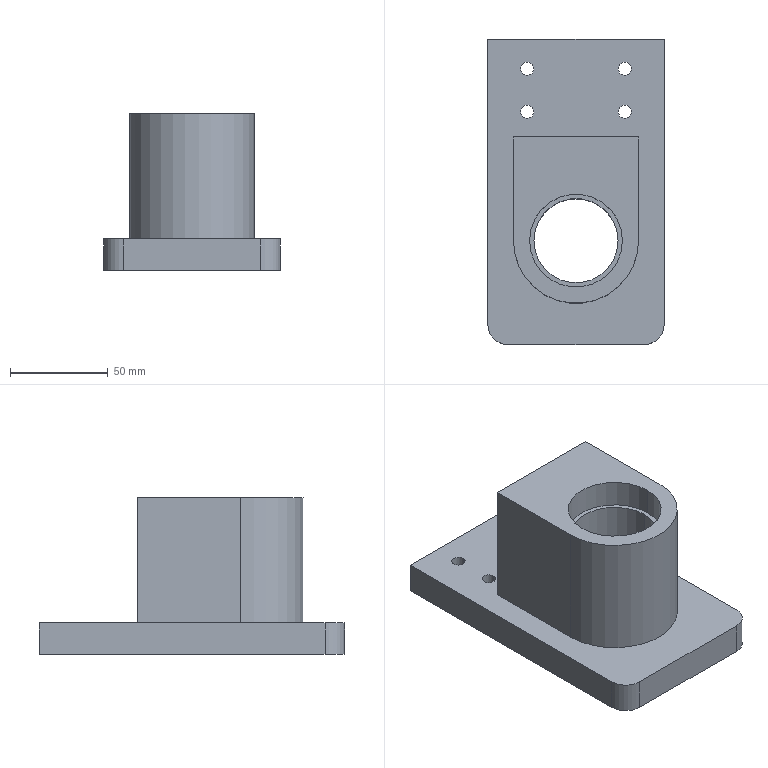NC program | NX | posted with a generic post | part box 90 x 156 x 80 mm
Lines 4809 to 4831 of 8711:
(PLANAR_MILL , TOOL : D50面刀)
N9616 T03 M6
N9618 G53
N9620 G17 G0 G90 X118. Y-10. S2000 M3
N9622 G43 Z30. H3
N9624 Z3.
N9626 G94 G1 Z0. F600.
N9628 X68.
N9630 X-78.
N9632 X-128.
N9634 Z3.
N9636 G0 Z30.
N9638 X118. Y20.
N9640 Z3.
N9642 G1 Z0.
N9644 X68.
N9646 X-78.
N9648 X-128.
N9650 Z3.
N9652 G0 Z30.
N9654 M5